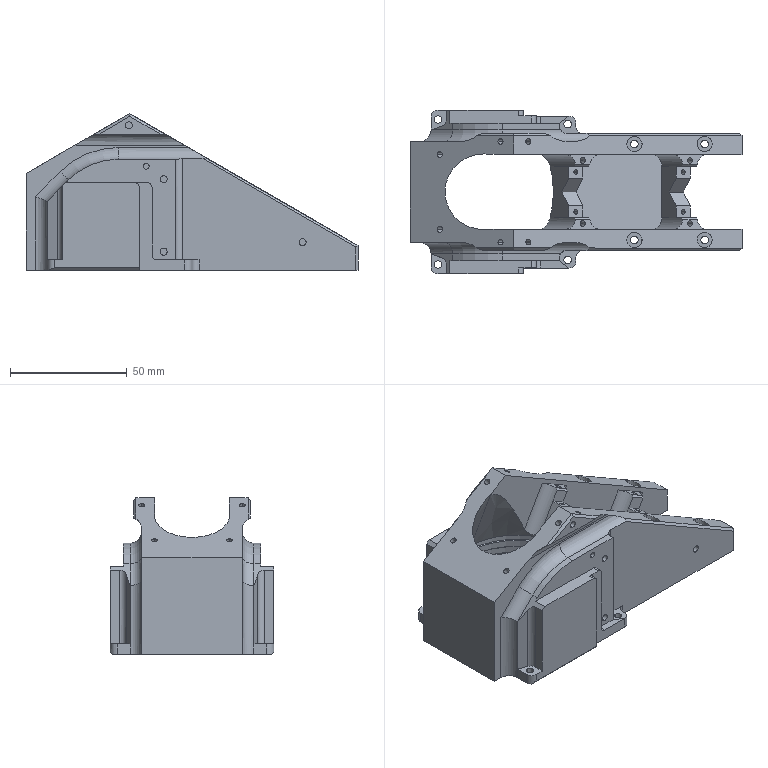NC program | NX | posted with a generic post | part box 142 x 70 x 67 mm
Lines 2969 to 4102 of 58889:
(PLANAR_MILL_COPY_COPY_COPY , TOOL : D6R0)
N5888 T04 M6
N5890 G54
N5892 G17 G0 G90 X-67.337 Y30.348 S3000 M3
N5894 G43 Z30. H4
N5896 G94 G1 Z-1. F5000.
N5898 G41 X-66.965 Y30.014 F1200. D4
N5900 G3 X-63.026 Y29.319 R4.
N5902 G1 X-58.5 Y30.966
N5904 Y35.
N5906 G3 X-60.5 Y38.464 R4.
N5908 G40
N5910 G1 X-60.941 Y38.699
N5912 G0 Z1.
N5914 X-67.337 Y30.348
N5916 G1 Z-2. F5000.
N5918 G41 X-66.965 Y30.014 F1200.
N5920 G3 X-63.026 Y29.319 R4.
N5922 G1 X-58.5 Y30.966
N5924 Y35.
N5926 G3 X-60.5 Y38.464 R4.
N5928 G40
N5930 G1 X-60.941 Y38.699
N5932 G0 Z0.
N5934 X-67.337 Y30.348
N5936 G1 Z-3. F5000.
N5938 G41 X-66.965 Y30.014 F1200.
N5940 G3 X-63.026 Y29.319 R4.
N5942 G1 X-58.5 Y30.966
N5944 Y35.
N5946 G3 X-60.5 Y38.464 R4.
N5948 G40
N5950 G1 X-60.941 Y38.699
N5952 G0 Z-1.
N5954 X-67.337 Y30.348
N5956 G1 Z-4. F5000.
N5958 G41 X-66.965 Y30.014 F1200.
N5960 G3 X-63.026 Y29.319 R4.
N5962 G1 X-58.5 Y30.966
N5964 Y35.
N5966 G3 X-60.5 Y38.464 R4.
N5968 G40
N5970 G1 X-60.941 Y38.699
N5972 G0 Z-2.
N5974 X-67.337 Y30.348
N5976 G1 Z-5. F5000.
N5978 G41 X-66.965 Y30.014 F1200.
N5980 G3 X-63.026 Y29.319 R4.
N5982 G1 X-58.5 Y30.966
N5984 Y35.
N5986 G3 X-60.5 Y38.464 R4.
N5988 G40
N5990 G1 X-60.941 Y38.699
N5992 G0 Z-3.
N5994 X-67.337 Y30.348
N5996 G1 Z-6. F5000.
N5998 G41 X-66.965 Y30.014 F1200.
N6000 G3 X-63.026 Y29.319 R4.
N6002 G1 X-58.5 Y30.966
N6004 Y35.
N6006 G3 X-60.5 Y38.464 R4.
N6008 G40
N6010 G1 X-60.941 Y38.699
N6012 G0 Z-4.
N6014 X-67.337 Y30.348
N6016 G1 Z-7. F5000.
N6018 G41 X-66.965 Y30.014 F1200.
N6020 G3 X-63.026 Y29.319 R4.
N6022 G1 X-58.5 Y30.966
N6024 Y35.
N6026 G3 X-60.5 Y38.464 R4.
N6028 G40
N6030 G1 X-60.941 Y38.699
N6032 G0 Z-5.
N6034 X-67.337 Y30.348
N6036 G1 Z-8. F5000.
N6038 G41 X-66.965 Y30.014 F1200.
N6040 G3 X-63.026 Y29.319 R4.
N6042 G1 X-58.5 Y30.966
N6044 Y35.
N6046 G3 X-60.5 Y38.464 R4.
N6048 G40
N6050 G1 X-60.941 Y38.699
N6052 G0 Z-6.
N6054 X-67.337 Y30.348
N6056 G1 Z-9. F5000.
N6058 G41 X-66.965 Y30.014 F1200.
N6060 G3 X-63.026 Y29.319 R4.
N6062 G1 X-58.5 Y30.966
N6064 Y35.
N6066 G3 X-60.5 Y38.464 R4.
N6068 G40
N6070 G1 X-60.941 Y38.699
N6072 G0 Z-7.
N6074 X-67.337 Y30.348
N6076 G1 Z-10. F5000.
N6078 G41 X-66.965 Y30.014 F1200.
N6080 G3 X-63.026 Y29.319 R4.
N6082 G1 X-58.5 Y30.966
N6084 Y35.
N6086 G3 X-60.5 Y38.464 R4.
N6088 G40
N6090 G1 X-60.941 Y38.699
N6092 G0 Z-8.
N6094 X-67.337 Y30.348
N6096 G1 Z-11. F5000.
N6098 G41 X-66.965 Y30.014 F1200.
N6100 G3 X-63.026 Y29.319 R4.
N6102 G1 X-58.5 Y30.966
N6104 Y35.
N6106 G3 X-60.5 Y38.464 R4.
N6108 G40
N6110 G1 X-60.941 Y38.699
N6112 G0 Z-9.
N6114 X-67.337 Y30.348
N6116 G1 Z-12. F5000.
N6118 G41 X-66.965 Y30.014 F1200.
N6120 G3 X-63.026 Y29.319 R4.
N6122 G1 X-58.5 Y30.966
N6124 Y35.
N6126 G3 X-60.5 Y38.464 R4.
N6128 G40
N6130 G1 X-60.941 Y38.699
N6132 G0 Z-10.
N6134 X-67.337 Y30.348
N6136 G1 Z-13. F5000.
N6138 G41 X-66.965 Y30.014 F1200.
N6140 G3 X-63.026 Y29.319 R4.
N6142 G1 X-58.5 Y30.966
N6144 Y35.
N6146 G3 X-60.5 Y38.464 R4.
N6148 G40
N6150 G1 X-60.941 Y38.699
N6152 G0 Z-11.
N6154 X-67.337 Y30.348
N6156 G1 Z-14. F5000.
N6158 G41 X-66.965 Y30.014 F1200.
N6160 G3 X-63.026 Y29.319 R4.
N6162 G1 X-58.5 Y30.966
N6164 Y35.
N6166 G3 X-60.5 Y38.464 R4.
N6168 G40
N6170 G1 X-60.941 Y38.699
N6172 G0 Z-12.
N6174 X-67.337 Y30.348
N6176 G1 Z-15. F5000.
N6178 G41 X-66.965 Y30.014 F1200.
N6180 G3 X-63.026 Y29.319 R4.
N6182 G1 X-58.5 Y30.966
N6184 Y35.
N6186 G3 X-60.5 Y38.464 R4.
N6188 G40
N6190 G1 X-60.941 Y38.699
N6192 G0 Z-13.
N6194 X-67.337 Y30.348
N6196 G1 Z-16. F5000.
N6198 G41 X-66.965 Y30.014 F1200.
N6200 G3 X-63.026 Y29.319 R4.
N6202 G1 X-58.5 Y30.966
N6204 Y35.
N6206 G3 X-60.5 Y38.464 R4.
N6208 G40
N6210 G1 X-60.941 Y38.699
N6212 G0 Z-14.
N6214 X-67.337 Y30.348
N6216 G1 Z-17. F5000.
N6218 G41 X-66.965 Y30.014 F1200.
N6220 G3 X-63.026 Y29.319 R4.
N6222 G1 X-58.5 Y30.966
N6224 Y35.
N6226 G3 X-60.5 Y38.464 R4.
N6228 G40
N6230 G1 X-60.941 Y38.699
N6232 G0 Z-15.
N6234 X-67.337 Y30.348
N6236 G1 Z-18. F5000.
N6238 G41 X-66.965 Y30.014 F1200.
N6240 G3 X-63.026 Y29.319 R4.
N6242 G1 X-58.5 Y30.966
N6244 Y35.
N6246 G3 X-60.5 Y38.464 R4.
N6248 G40
N6250 G1 X-60.941 Y38.699
N6252 G0 Z-16.
N6254 X-67.337 Y30.348
N6256 G1 Z-19. F5000.
N6258 G41 X-66.965 Y30.014 F1200.
N6260 G3 X-63.026 Y29.319 R4.
N6262 G1 X-58.5 Y30.966
N6264 Y35.
N6266 G3 X-60.5 Y38.464 R4.
N6268 G40
N6270 G1 X-60.941 Y38.699
N6272 G0 Z-17.
N6274 X-67.337 Y30.348
N6276 G1 Z-20. F5000.
N6278 G41 X-66.965 Y30.014 F1200.
N6280 G3 X-63.026 Y29.319 R4.
N6282 G1 X-58.5 Y30.966
N6284 Y35.
N6286 G3 X-60.5 Y38.464 R4.
N6288 G40
N6290 G1 X-60.941 Y38.699
N6292 G0 Z-18.
N6294 X-67.337 Y30.348
N6296 G1 Z-21. F5000.
N6298 G41 X-66.965 Y30.014 F1200.
N6300 G3 X-63.026 Y29.319 R4.
N6302 G1 X-58.5 Y30.966
N6304 Y35.
N6306 G3 X-60.5 Y38.464 R4.
N6308 G40
N6310 G1 X-60.941 Y38.699
N6312 G0 Z-19.
N6314 X-67.337 Y30.348
N6316 G1 Z-22. F5000.
N6318 G41 X-66.965 Y30.014 F1200.
N6320 G3 X-63.026 Y29.319 R4.
N6322 G1 X-58.5 Y30.966
N6324 Y35.
N6326 G3 X-60.5 Y38.464 R4.
N6328 G40
N6330 G1 X-60.941 Y38.699
N6332 G0 Z-20.
N6334 X-67.337 Y30.348
N6336 G1 Z-23. F5000.
N6338 G41 X-66.965 Y30.014 F1200.
N6340 G3 X-63.026 Y29.319 R4.
N6342 G1 X-58.5 Y30.966
N6344 Y35.
N6346 G3 X-60.5 Y38.464 R4.
N6348 G40
N6350 G1 X-60.941 Y38.699
N6352 G0 Z-21.
N6354 X-67.337 Y30.348
N6356 G1 Z-24. F5000.
N6358 G41 X-66.965 Y30.014 F1200.
N6360 G3 X-63.026 Y29.319 R4.
N6362 G1 X-58.5 Y30.966
N6364 Y35.
N6366 G3 X-60.5 Y38.464 R4.
N6368 G40
N6370 G1 X-60.941 Y38.699
N6372 G0 Z-22.
N6374 X-67.337 Y30.348
N6376 G1 Z-25. F5000.
N6378 G41 X-66.965 Y30.014 F1200.
N6380 G3 X-63.026 Y29.319 R4.
N6382 G1 X-58.5 Y30.966
N6384 Y35.
N6386 G3 X-60.5 Y38.464 R4.
N6388 G40
N6390 G1 X-60.941 Y38.699
N6392 G0 Z-23.
N6394 X-67.337 Y30.348
N6396 G1 Z-26. F5000.
N6398 G41 X-66.965 Y30.014 F1200.
N6400 G3 X-63.026 Y29.319 R4.
N6402 G1 X-58.5 Y30.966
N6404 Y35.
N6406 G3 X-60.5 Y38.464 R4.
N6408 G40
N6410 G1 X-60.941 Y38.699
N6412 G0 Z-24.
N6414 X-67.337 Y30.348
N6416 G1 Z-27. F5000.
N6418 G41 X-66.965 Y30.014 F1200.
N6420 G3 X-63.026 Y29.319 R4.
N6422 G1 X-58.5 Y30.966
N6424 Y35.
N6426 G3 X-60.5 Y38.464 R4.
N6428 G40
N6430 G1 X-60.941 Y38.699
N6432 G0 Z-25.
N6434 X-67.337 Y30.348
N6436 G1 Z-28. F5000.
N6438 G41 X-66.965 Y30.014 F1200.
N6440 G3 X-63.026 Y29.319 R4.
N6442 G1 X-58.5 Y30.966
N6444 Y35.
N6446 G3 X-60.5 Y38.464 R4.
N6448 G40
N6450 G1 X-60.941 Y38.699
N6452 G0 Z-26.
N6454 X-67.337 Y30.348
N6456 G1 Z-29. F5000.
N6458 G41 X-66.965 Y30.014 F1200.
N6460 G3 X-63.026 Y29.319 R4.
N6462 G1 X-58.5 Y30.966
N6464 Y35.
N6466 G3 X-60.5 Y38.464 R4.
N6468 G40
N6470 G1 X-60.941 Y38.699
N6472 G0 Z-27.
N6474 X-67.337 Y30.348
N6476 G1 Z-30. F5000.
N6478 G41 X-66.965 Y30.014 F1200.
N6480 G3 X-63.026 Y29.319 R4.
N6482 G1 X-58.5 Y30.966
N6484 Y35.
N6486 G3 X-60.5 Y38.464 R4.
N6488 G40
N6490 G1 X-60.941 Y38.699
N6492 G0 Z-28.
N6494 X-67.337 Y30.348
N6496 G1 Z-31. F5000.
N6498 G41 X-66.965 Y30.014 F1200.
N6500 G3 X-63.026 Y29.319 R4.
N6502 G1 X-58.5 Y30.966
N6504 Y35.
N6506 G3 X-60.5 Y38.464 R4.
N6508 G40
N6510 G1 X-60.941 Y38.699
N6512 G0 Z-29.
N6514 X-67.337 Y30.348
N6516 G1 Z-32. F5000.
N6518 G41 X-66.965 Y30.014 F1200.
N6520 G3 X-63.026 Y29.319 R4.
N6522 G1 X-58.5 Y30.966
N6524 Y35.
N6526 G3 X-60.5 Y38.464 R4.
N6528 G40
N6530 G1 X-60.941 Y38.699
N6532 G0 Z-30.
N6534 X-67.337 Y30.348
N6536 G1 Z-33. F5000.
N6538 G41 X-66.965 Y30.014 F1200.
N6540 G3 X-63.026 Y29.319 R4.
N6542 G1 X-58.5 Y30.966
N6544 Y35.
N6546 G3 X-60.5 Y38.464 R4.
N6548 G40
N6550 G1 X-60.941 Y38.699
N6552 G0 Z-31.
N6554 X-67.337 Y30.348
N6556 G1 Z-34. F5000.
N6558 G41 X-66.965 Y30.014 F1200.
N6560 G3 X-63.026 Y29.319 R4.
N6562 G1 X-58.5 Y30.966
N6564 Y35.
N6566 G3 X-60.5 Y38.464 R4.
N6568 G40
N6570 G1 X-60.941 Y38.699
N6572 G0 Z-32.
N6574 X-67.337 Y30.348
N6576 G1 Z-35. F5000.
N6578 G41 X-66.965 Y30.014 F1200.
N6580 G3 X-63.026 Y29.319 R4.
N6582 G1 X-58.5 Y30.966
N6584 Y35.
N6586 G3 X-60.5 Y38.464 R4.
N6588 G40
N6590 G1 X-60.941 Y38.699
N6592 G0 Z-33.
N6594 X-67.337 Y30.348
N6596 G1 Z-36. F5000.
N6598 G41 X-66.965 Y30.014 F1200.
N6600 G3 X-63.026 Y29.319 R4.
N6602 G1 X-58.5 Y30.966
N6604 Y35.
N6606 G3 X-60.5 Y38.464 R4.
N6608 G40
N6610 G1 X-60.941 Y38.699
N6612 G0 Z-34.
N6614 X-67.337 Y30.348
N6616 G1 Z-37. F5000.
N6618 G41 X-66.965 Y30.014 F1200.
N6620 G3 X-63.026 Y29.319 R4.
N6622 G1 X-58.5 Y30.966
N6624 Y35.
N6626 G3 X-60.5 Y38.464 R4.
N6628 G40
N6630 G1 X-60.941 Y38.699
N6632 G0 Z-35.
N6634 X-67.337 Y30.348
N6636 G1 Z-38. F5000.
N6638 G41 X-66.965 Y30.014 F1200.
N6640 G3 X-63.026 Y29.319 R4.
N6642 G1 X-58.5 Y30.966
N6644 Y35.
N6646 G3 X-60.5 Y38.464 R4.
N6648 G40
N6650 G1 X-60.941 Y38.699
N6652 G0 Z-36.
N6654 X-67.337 Y30.348
N6656 G1 Z-39. F5000.
N6658 G41 X-66.965 Y30.014 F1200.
N6660 G3 X-63.026 Y29.319 R4.
N6662 G1 X-58.5 Y30.966
N6664 Y35.
N6666 G3 X-60.5 Y38.464 R4.
N6668 G40
N6670 G1 X-60.941 Y38.699
N6672 G0 Z-37.
N6674 X-67.337 Y30.348
N6676 G1 Z-40. F5000.
N6678 G41 X-66.965 Y30.014 F1200.
N6680 G3 X-63.026 Y29.319 R4.
N6682 G1 X-58.5 Y30.966
N6684 Y35.
N6686 G3 X-60.5 Y38.464 R4.
N6688 G40
N6690 G1 X-60.941 Y38.699
N6692 G0 Z-38.
N6694 X-67.337 Y30.348
N6696 G1 Z-41. F5000.
N6698 G41 X-66.965 Y30.014 F1200.
N6700 G3 X-63.026 Y29.319 R4.
N6702 G1 X-58.5 Y30.966
N6704 Y35.
N6706 G3 X-60.5 Y38.464 R4.
N6708 G40
N6710 G1 X-60.941 Y38.699
N6712 G0 Z-39.
N6714 X-67.337 Y30.348
N6716 G1 Z-42. F5000.
N6718 G41 X-66.965 Y30.014 F1200.
N6720 G3 X-63.026 Y29.319 R4.
N6722 G1 X-58.5 Y30.966
N6724 Y35.
N6726 G3 X-60.5 Y38.464 R4.
N6728 G40
N6730 G1 X-60.941 Y38.699
N6732 G0 Z-40.
N6734 X-67.337 Y30.348
N6736 G1 Z-43. F5000.
N6738 G41 X-66.965 Y30.014 F1200.
N6740 G3 X-63.026 Y29.319 R4.
N6742 G1 X-58.5 Y30.966
N6744 Y35.
N6746 G3 X-60.5 Y38.464 R4.
N6748 G40
N6750 G1 X-60.941 Y38.699
N6752 G0 Z-41.
N6754 X-67.337 Y30.348
N6756 G1 Z-44. F5000.
N6758 G41 X-66.965 Y30.014 F1200.
N6760 G3 X-63.026 Y29.319 R4.
N6762 G1 X-58.5 Y30.966
N6764 Y35.
N6766 G3 X-60.5 Y38.464 R4.
N6768 G40
N6770 G1 X-60.941 Y38.699
N6772 G0 Z-42.
N6774 X-67.337 Y30.348
N6776 G1 Z-45. F5000.
N6778 G41 X-66.965 Y30.014 F1200.
N6780 G3 X-63.026 Y29.319 R4.
N6782 G1 X-58.5 Y30.966
N6784 Y35.
N6786 G3 X-60.5 Y38.464 R4.
N6788 G40
N6790 G1 X-60.941 Y38.699
N6792 G0 Z-43.
N6794 X-67.337 Y30.348
N6796 G1 Z-46. F5000.
N6798 G41 X-66.965 Y30.014 F1200.
N6800 G3 X-63.026 Y29.319 R4.
N6802 G1 X-58.5 Y30.966
N6804 Y35.
N6806 G3 X-60.5 Y38.464 R4.
N6808 G40
N6810 G1 X-60.941 Y38.699
N6812 G0 Z-44.
N6814 X-67.337 Y30.348
N6816 G1 Z-47. F5000.
N6818 G41 X-66.965 Y30.014 F1200.
N6820 G3 X-63.026 Y29.319 R4.
N6822 G1 X-58.5 Y30.966
N6824 Y35.
N6826 G3 X-60.5 Y38.464 R4.
N6828 G40
N6830 G1 X-60.941 Y38.699
N6832 G0 Z-45.
N6834 X-67.337 Y30.348
N6836 G1 Z-48. F5000.
N6838 G41 X-66.965 Y30.014 F1200.
N6840 G3 X-63.026 Y29.319 R4.
N6842 G1 X-58.5 Y30.966
N6844 Y35.
N6846 G3 X-60.5 Y38.464 R4.
N6848 G40
N6850 G1 X-60.941 Y38.699
N6852 G0 Z-46.
N6854 X-67.337 Y30.348
N6856 G1 Z-49. F5000.
N6858 G41 X-66.965 Y30.014 F1200.
N6860 G3 X-63.026 Y29.319 R4.
N6862 G1 X-58.5 Y30.966
N6864 Y35.
N6866 G3 X-60.5 Y38.464 R4.
N6868 G40
N6870 G1 X-60.941 Y38.699
N6872 G0 Z-47.
N6874 X-67.337 Y30.348
N6876 G1 Z-50. F5000.
N6878 G41 X-66.965 Y30.014 F1200.
N6880 G3 X-63.026 Y29.319 R4.
N6882 G1 X-58.5 Y30.966
N6884 Y35.
N6886 G3 X-60.5 Y38.464 R4.
N6888 G40
N6890 G1 X-60.941 Y38.699
N6892 G0 Z-48.
N6894 X-67.337 Y30.348
N6896 G1 Z-51. F5000.
N6898 G41 X-66.965 Y30.014 F1200.
N6900 G3 X-63.026 Y29.319 R4.
N6902 G1 X-58.5 Y30.966
N6904 Y35.
N6906 G3 X-60.5 Y38.464 R4.
N6908 G40
N6910 G1 X-60.941 Y38.699
N6912 G0 Z-49.
N6914 X-67.337 Y30.348
N6916 G1 Z-52. F5000.
N6918 G41 X-66.965 Y30.014 F1200.
N6920 G3 X-63.026 Y29.319 R4.
N6922 G1 X-58.5 Y30.966
N6924 Y35.
N6926 G3 X-60.5 Y38.464 R4.
N6928 G40
N6930 G1 X-60.941 Y38.699
N6932 G0 Z-50.
N6934 X-67.337 Y30.348
N6936 G1 Z-53. F5000.
N6938 G41 X-66.965 Y30.014 F1200.
N6940 G3 X-63.026 Y29.319 R4.
N6942 G1 X-58.5 Y30.966
N6944 Y35.
N6946 G3 X-60.5 Y38.464 R4.
N6948 G40
N6950 G1 X-60.941 Y38.699
N6952 G0 Z-51.
N6954 X-67.337 Y30.348
N6956 G1 Z-54. F5000.
N6958 G41 X-66.965 Y30.014 F1200.
N6960 G3 X-63.026 Y29.319 R4.
N6962 G1 X-58.5 Y30.966
N6964 Y35.
N6966 G3 X-60.5 Y38.464 R4.
N6968 G40
N6970 G1 X-60.941 Y38.699
N6972 G0 Z-52.
N6974 X-67.337 Y30.348
N6976 G1 Z-55. F5000.
N6978 G41 X-66.965 Y30.014 F1200.
N6980 G3 X-63.026 Y29.319 R4.
N6982 G1 X-58.5 Y30.966
N6984 Y35.
N6986 G3 X-60.5 Y38.464 R4.
N6988 G40
N6990 G1 X-60.941 Y38.699
N6992 G0 Z-53.
N6994 X-67.337 Y30.348
N6996 G1 Z-56. F5000.
N6998 G41 X-66.965 Y30.014 F1200.
N7000 G3 X-63.026 Y29.319 R4.
N7002 G1 X-58.5 Y30.966
N7004 Y35.
N7006 G3 X-60.5 Y38.464 R4.
N7008 G40
N7010 G1 X-60.941 Y38.699
N7012 G0 Z-54.
N7014 X-67.337 Y30.348
N7016 G1 Z-57. F5000.
N7018 G41 X-66.965 Y30.014 F1200.
N7020 G3 X-63.026 Y29.319 R4.
N7022 G1 X-58.5 Y30.966
N7024 Y35.
N7026 G3 X-60.5 Y38.464 R4.
N7028 G40
N7030 G1 X-60.941 Y38.699
N7032 G0 Z-55.
N7034 X-67.337 Y30.348
N7036 G1 Z-58. F5000.
N7038 G41 X-66.965 Y30.014 F1200.
N7040 G3 X-63.026 Y29.319 R4.
N7042 G1 X-58.5 Y30.966
N7044 Y35.
N7046 G3 X-60.5 Y38.464 R4.
N7048 G40
N7050 G1 X-60.941 Y38.699
N7052 G0 Z-56.
N7054 X-67.337 Y30.348
N7056 G1 Z-59. F5000.
N7058 G41 X-66.965 Y30.014 F1200.
N7060 G3 X-63.026 Y29.319 R4.
N7062 G1 X-58.5 Y30.966
N7064 Y35.
N7066 G3 X-60.5 Y38.464 R4.
N7068 G40
N7070 G1 X-60.941 Y38.699
N7072 G0 Z-57.
N7074 X-67.337 Y30.348
N7076 G1 Z-60. F5000.
N7078 G41 X-66.965 Y30.014 F1200.
N7080 G3 X-63.026 Y29.319 R4.
N7082 G1 X-58.5 Y30.966
N7084 Y35.
N7086 G3 X-60.5 Y38.464 R4.
N7088 G40
N7090 G1 X-60.941 Y38.699
N7092 G0 Z-58.
N7094 X-67.337 Y30.348
N7096 G1 Z-61. F5000.
N7098 G41 X-66.965 Y30.014 F1200.
N7100 G3 X-63.026 Y29.319 R4.
N7102 G1 X-58.5 Y30.966
N7104 Y35.
N7106 G3 X-60.5 Y38.464 R4.
N7108 G40
N7110 G1 X-60.941 Y38.699
N7112 G0 Z-59.
N7114 X-67.337 Y30.348
N7116 G1 Z-62. F5000.
N7118 G41 X-66.965 Y30.014 F1200.
N7120 G3 X-63.026 Y29.319 R4.
N7122 G1 X-58.5 Y30.966
N7124 Y35.
N7126 G3 X-60.5 Y38.464 R4.
N7128 G40
N7130 G1 X-60.941 Y38.699
N7132 G0 Z-60.
N7134 X-67.337 Y30.348
N7136 G1 Z-62.5 F5000.
N7138 G41 X-66.965 Y30.014 F1200.
N7140 G3 X-63.026 Y29.319 R4.
N7142 G1 X-58.5 Y30.966
N7144 Y35.
N7146 G3 X-60.5 Y38.464 R4.
N7148 G40
N7150 G1 X-60.941 Y38.699
N7152 G0 Z30.
N7154 X-1.659 Y36.199
N7156 G1 Z-1. F5000.
N7158 G41 X-2.1 Y35.964 F1200.
N7160 G3 X-4.1 Y32.5 R4.
N7162 G1 Y28.
N7164 X4.
N7166 G3 X7.464 Y30. R4.
N7168 G40
N7170 G1 X7.699 Y30.441
N7172 G0 Z1.
N7174 X-1.659 Y36.199
N7176 G1 Z-2. F5000.
N7178 G41 X-2.1 Y35.964 F1200.
N7180 G3 X-4.1 Y32.5 R4.
N7182 G1 Y28.
N7184 X4.
N7186 G3 X7.464 Y30. R4.
N7188 G40
N7190 G1 X7.699 Y30.441
N7192 G0 Z0.
N7194 X-1.659 Y36.199
N7196 G1 Z-3. F5000.
N7198 G41 X-2.1 Y35.964 F1200.
N7200 G3 X-4.1 Y32.5 R4.
N7202 G1 Y28.
N7204 X4.
N7206 G3 X7.464 Y30. R4.
N7208 G40
N7210 G1 X7.699 Y30.441
N7212 G0 Z-1.
N7214 X-1.659 Y36.199
N7216 G1 Z-4. F5000.
N7218 G41 X-2.1 Y35.964 F1200.
N7220 G3 X-4.1 Y32.5 R4.
N7222 G1 Y28.
N7224 X4.
N7226 G3 X7.464 Y30. R4.
N7228 G40
N7230 G1 X7.699 Y30.441
N7232 G0 Z-2.
N7234 X-1.659 Y36.199
N7236 G1 Z-5. F5000.
N7238 G41 X-2.1 Y35.964 F1200.
N7240 G3 X-4.1 Y32.5 R4.
N7242 G1 Y28.
N7244 X4.
N7246 G3 X7.464 Y30. R4.
N7248 G40
N7250 G1 X7.699 Y30.441
N7252 G0 Z-3.
N7254 X-1.659 Y36.199
N7256 G1 Z-6. F5000.
N7258 G41 X-2.1 Y35.964 F1200.
N7260 G3 X-4.1 Y32.5 R4.
N7262 G1 Y28.
N7264 X4.
N7266 G3 X7.464 Y30. R4.
N7268 G40
N7270 G1 X7.699 Y30.441
N7272 G0 Z-4.
N7274 X-1.659 Y36.199
N7276 G1 Z-7. F5000.
N7278 G41 X-2.1 Y35.964 F1200.
N7280 G3 X-4.1 Y32.5 R4.
N7282 G1 Y28.
N7284 X4.
N7286 G3 X7.464 Y30. R4.
N7288 G40
N7290 G1 X7.699 Y30.441
N7292 G0 Z-5.
N7294 X-1.659 Y36.199
N7296 G1 Z-8. F5000.
N7298 G41 X-2.1 Y35.964 F1200.
N7300 G3 X-4.1 Y32.5 R4.
N7302 G1 Y28.
N7304 X4.
N7306 G3 X7.464 Y30. R4.
N7308 G40
N7310 G1 X7.699 Y30.441
N7312 G0 Z-6.
N7314 X-1.659 Y36.199
N7316 G1 Z-9. F5000.
N7318 G41 X-2.1 Y35.964 F1200.
N7320 G3 X-4.1 Y32.5 R4.
N7322 G1 Y28.
N7324 X4.
N7326 G3 X7.464 Y30. R4.
N7328 G40
N7330 G1 X7.699 Y30.441
N7332 G0 Z-7.
N7334 X-1.659 Y36.199
N7336 G1 Z-10. F5000.
N7338 G41 X-2.1 Y35.964 F1200.
N7340 G3 X-4.1 Y32.5 R4.
N7342 G1 Y28.
N7344 X4.
N7346 G3 X7.464 Y30. R4.
N7348 G40
N7350 G1 X7.699 Y30.441
N7352 G0 Z-8.
N7354 X-1.659 Y36.199
N7356 G1 Z-11. F5000.
N7358 G41 X-2.1 Y35.964 F1200.
N7360 G3 X-4.1 Y32.5 R4.
N7362 G1 Y28.
N7364 X4.
N7366 G3 X7.464 Y30. R4.
N7368 G40
N7370 G1 X7.699 Y30.441
N7372 G0 Z-9.
N7374 X-1.659 Y36.199
N7376 G1 Z-12. F5000.
N7378 G41 X-2.1 Y35.964 F1200.
N7380 G3 X-4.1 Y32.5 R4.
N7382 G1 Y28.
N7384 X4.
N7386 G3 X7.464 Y30. R4.
N7388 G40
N7390 G1 X7.699 Y30.441
N7392 G0 Z-10.
N7394 X-1.659 Y36.199
N7396 G1 Z-13. F5000.
N7398 G41 X-2.1 Y35.964 F1200.
N7400 G3 X-4.1 Y32.5 R4.
N7402 G1 Y28.
N7404 X4.
N7406 G3 X7.464 Y30. R4.
N7408 G40
N7410 G1 X7.699 Y30.441
N7412 G0 Z-11.
N7414 X-1.659 Y36.199
N7416 G1 Z-14. F5000.
N7418 G41 X-2.1 Y35.964 F1200.
N7420 G3 X-4.1 Y32.5 R4.
N7422 G1 Y28.
N7424 X4.
N7426 G3 X7.464 Y30. R4.
N7428 G40
N7430 G1 X7.699 Y30.441
N7432 G0 Z-12.
N7434 X-1.659 Y36.199
N7436 G1 Z-15. F5000.
N7438 G41 X-2.1 Y35.964 F1200.
N7440 G3 X-4.1 Y32.5 R4.
N7442 G1 Y28.
N7444 X4.
N7446 G3 X7.464 Y30. R4.
N7448 G40
N7450 G1 X7.699 Y30.441
N7452 G0 Z-13.
N7454 X-1.659 Y36.199
N7456 G1 Z-16. F5000.
N7458 G41 X-2.1 Y35.964 F1200.
N7460 G3 X-4.1 Y32.5 R4.
N7462 G1 Y28.
N7464 X4.
N7466 G3 X7.464 Y30. R4.
N7468 G40
N7470 G1 X7.699 Y30.441
N7472 G0 Z-14.
N7474 X-1.659 Y36.199
N7476 G1 Z-17. F5000.
N7478 G41 X-2.1 Y35.964 F1200.
N7480 G3 X-4.1 Y32.5 R4.
N7482 G1 Y28.
N7484 X4.
N7486 G3 X7.464 Y30. R4.
N7488 G40
N7490 G1 X7.699 Y30.441
N7492 G0 Z-15.
N7494 X-1.659 Y36.199
N7496 G1 Z-18. F5000.
N7498 G41 X-2.1 Y35.964 F1200.
N7500 G3 X-4.1 Y32.5 R4.
N7502 G1 Y28.
N7504 X4.
N7506 G3 X7.464 Y30. R4.
N7508 G40
N7510 G1 X7.699 Y30.441
N7512 G0 Z-16.
N7514 X-1.659 Y36.199
N7516 G1 Z-19. F5000.
N7518 G41 X-2.1 Y35.964 F1200.
N7520 G3 X-4.1 Y32.5 R4.
N7522 G1 Y28.
N7524 X4.
N7526 G3 X7.464 Y30. R4.
N7528 G40
N7530 G1 X7.699 Y30.441
N7532 G0 Z-17.
N7534 X-1.659 Y36.199
N7536 G1 Z-20. F5000.
N7538 G41 X-2.1 Y35.964 F1200.
N7540 G3 X-4.1 Y32.5 R4.
N7542 G1 Y28.
N7544 X4.
N7546 G3 X7.464 Y30. R4.
N7548 G40
N7550 G1 X7.699 Y30.441
N7552 G0 Z-18.
N7554 X-1.659 Y36.199
N7556 G1 Z-21. F5000.
N7558 G41 X-2.1 Y35.964 F1200.
N7560 G3 X-4.1 Y32.5 R4.
N7562 G1 Y28.
N7564 X4.
N7566 G3 X7.464 Y30. R4.
N7568 G40
N7570 G1 X7.699 Y30.441
N7572 G0 Z-19.
N7574 X-1.659 Y36.199
N7576 G1 Z-22. F5000.
N7578 G41 X-2.1 Y35.964 F1200.
N7580 G3 X-4.1 Y32.5 R4.
N7582 G1 Y28.
N7584 X4.
N7586 G3 X7.464 Y30. R4.
N7588 G40
N7590 G1 X7.699 Y30.441
N7592 G0 Z-20.
N7594 X-1.659 Y36.199
N7596 G1 Z-23. F5000.
N7598 G41 X-2.1 Y35.964 F1200.
N7600 G3 X-4.1 Y32.5 R4.
N7602 G1 Y28.
N7604 X4.
N7606 G3 X7.464 Y30. R4.
N7608 G40
N7610 G1 X7.699 Y30.441
N7612 G0 Z-21.
N7614 X-1.659 Y36.199
N7616 G1 Z-24. F5000.
N7618 G41 X-2.1 Y35.964 F1200.
N7620 G3 X-4.1 Y32.5 R4.
N7622 G1 Y28.
N7624 X4.
N7626 G3 X7.464 Y30. R4.
N7628 G40
N7630 G1 X7.699 Y30.441
N7632 G0 Z-22.
N7634 X-1.659 Y36.199
N7636 G1 Z-25. F5000.
N7638 G41 X-2.1 Y35.964 F1200.
N7640 G3 X-4.1 Y32.5 R4.
N7642 G1 Y28.
N7644 X4.
N7646 G3 X7.464 Y30. R4.
N7648 G40
N7650 G1 X7.699 Y30.441
N7652 G0 Z-23.
N7654 X-1.659 Y36.199
N7656 G1 Z-26. F5000.
N7658 G41 X-2.1 Y35.964 F1200.
N7660 G3 X-4.1 Y32.5 R4.
N7662 G1 Y28.
N7664 X4.
N7666 G3 X7.464 Y30. R4.
N7668 G40
N7670 G1 X7.699 Y30.441
N7672 G0 Z-24.
N7674 X-1.659 Y36.199
N7676 G1 Z-27. F5000.
N7678 G41 X-2.1 Y35.964 F1200.
N7680 G3 X-4.1 Y32.5 R4.
N7682 G1 Y28.
N7684 X4.
N7686 G3 X7.464 Y30. R4.
N7688 G40
N7690 G1 X7.699 Y30.441
N7692 G0 Z-25.
N7694 X-1.659 Y36.199
N7696 G1 Z-28. F5000.
N7698 G41 X-2.1 Y35.964 F1200.
N7700 G3 X-4.1 Y32.5 R4.
N7702 G1 Y28.
N7704 X4.
N7706 G3 X7.464 Y30. R4.
N7708 G40
N7710 G1 X7.699 Y30.441
N7712 G0 Z-26.
N7714 X-1.659 Y36.199
N7716 G1 Z-29. F5000.
N7718 G41 X-2.1 Y35.964 F1200.
N7720 G3 X-4.1 Y32.5 R4.
N7722 G1 Y28.
N7724 X4.
N7726 G3 X7.464 Y30. R4.
N7728 G40
N7730 G1 X7.699 Y30.441
N7732 G0 Z-27.
N7734 X-1.659 Y36.199
N7736 G1 Z-30. F5000.
N7738 G41 X-2.1 Y35.964 F1200.
N7740 G3 X-4.1 Y32.5 R4.
N7742 G1 Y28.
N7744 X4.
N7746 G3 X7.464 Y30. R4.
N7748 G40
N7750 G1 X7.699 Y30.441
N7752 G0 Z-28.
N7754 X-1.659 Y36.199
N7756 G1 Z-31. F5000.
N7758 G41 X-2.1 Y35.964 F1200.
N7760 G3 X-4.1 Y32.5 R4.
N7762 G1 Y28.
N7764 X4.
N7766 G3 X7.464 Y30. R4.
N7768 G40
N7770 G1 X7.699 Y30.441
N7772 G0 Z-29.
N7774 X-1.659 Y36.199
N7776 G1 Z-32. F5000.
N7778 G41 X-2.1 Y35.964 F1200.
N7780 G3 X-4.1 Y32.5 R4.
N7782 G1 Y28.
N7784 X4.
N7786 G3 X7.464 Y30. R4.
N7788 G40
N7790 G1 X7.699 Y30.441
N7792 G0 Z-30.
N7794 X-1.659 Y36.199
N7796 G1 Z-33. F5000.
N7798 G41 X-2.1 Y35.964 F1200.
N7800 G3 X-4.1 Y32.5 R4.
N7802 G1 Y28.
N7804 X4.
N7806 G3 X7.464 Y30. R4.
N7808 G40
N7810 G1 X7.699 Y30.441
N7812 G0 Z-31.
N7814 X-1.659 Y36.199
N7816 G1 Z-34. F5000.
N7818 G41 X-2.1 Y35.964 F1200.
N7820 G3 X-4.1 Y32.5 R4.
N7822 G1 Y28.
N7824 X4.
N7826 G3 X7.464 Y30. R4.
N7828 G40
N7830 G1 X7.699 Y30.441
N7832 G0 Z-32.
N7834 X-1.659 Y36.199
N7836 G1 Z-35. F5000.
N7838 G41 X-2.1 Y35.964 F1200.
N7840 G3 X-4.1 Y32.5 R4.
N7842 G1 Y28.
N7844 X4.
N7846 G3 X7.464 Y30. R4.
N7848 G40
N7850 G1 X7.699 Y30.441
N7852 G0 Z-33.
N7854 X-1.659 Y36.199
N7856 G1 Z-36. F5000.
N7858 G41 X-2.1 Y35.964 F1200.
N7860 G3 X-4.1 Y32.5 R4.
N7862 G1 Y28.
N7864 X4.
N7866 G3 X7.464 Y30. R4.
N7868 G40
N7870 G1 X7.699 Y30.441
N7872 G0 Z-34.
N7874 X-1.659 Y36.199
N7876 G1 Z-37. F5000.
N7878 G41 X-2.1 Y35.964 F1200.
N7880 G3 X-4.1 Y32.5 R4.
N7882 G1 Y28.
N7884 X4.
N7886 G3 X7.464 Y30. R4.
N7888 G40
N7890 G1 X7.699 Y30.441
N7892 G0 Z-35.
N7894 X-1.659 Y36.199
N7896 G1 Z-38. F5000.
N7898 G41 X-2.1 Y35.964 F1200.
N7900 G3 X-4.1 Y32.5 R4.
N7902 G1 Y28.
N7904 X4.
N7906 G3 X7.464 Y30. R4.
N7908 G40
N7910 G1 X7.699 Y30.441
N7912 G0 Z-36.
N7914 X-1.659 Y36.199
N7916 G1 Z-39. F5000.
N7918 G41 X-2.1 Y35.964 F1200.
N7920 G3 X-4.1 Y32.5 R4.
N7922 G1 Y28.
N7924 X4.
N7926 G3 X7.464 Y30. R4.
N7928 G40
N7930 G1 X7.699 Y30.441
N7932 G0 Z-37.
N7934 X-1.659 Y36.199
N7936 G1 Z-40. F5000.
N7938 G41 X-2.1 Y35.964 F1200.
N7940 G3 X-4.1 Y32.5 R4.
N7942 G1 Y28.
N7944 X4.
N7946 G3 X7.464 Y30. R4.
N7948 G40
N7950 G1 X7.699 Y30.441
N7952 G0 Z-38.
N7954 X-1.659 Y36.199
N7956 G1 Z-41. F5000.
N7958 G41 X-2.1 Y35.964 F1200.
N7960 G3 X-4.1 Y32.5 R4.
N7962 G1 Y28.
N7964 X4.
N7966 G3 X7.464 Y30. R4.
N7968 G40
N7970 G1 X7.699 Y30.441
N7972 G0 Z-39.
N7974 X-1.659 Y36.199
N7976 G1 Z-42. F5000.
N7978 G41 X-2.1 Y35.964 F1200.
N7980 G3 X-4.1 Y32.5 R4.
N7982 G1 Y28.
N7984 X4.
N7986 G3 X7.464 Y30. R4.
N7988 G40
N7990 G1 X7.699 Y30.441
N7992 G0 Z-40.
N7994 X-1.659 Y36.199
N7996 G1 Z-43. F5000.
N7998 G41 X-2.1 Y35.964 F1200.
N8000 G3 X-4.1 Y32.5 R4.
N8002 G1 Y28.
N8004 X4.
N8006 G3 X7.464 Y30. R4.
N8008 G40
N8010 G1 X7.699 Y30.441
N8012 G0 Z-41.
N8014 X-1.659 Y36.199
N8016 G1 Z-44. F5000.
N8018 G41 X-2.1 Y35.964 F1200.
N8020 G3 X-4.1 Y32.5 R4.
N8022 G1 Y28.
N8024 X4.
N8026 G3 X7.464 Y30. R4.
N8028 G40
N8030 G1 X7.699 Y30.441
N8032 G0 Z-42.
N8034 X-1.659 Y36.199
N8036 G1 Z-45. F5000.
N8038 G41 X-2.1 Y35.964 F1200.
N8040 G3 X-4.1 Y32.5 R4.
N8042 G1 Y28.
N8044 X4.
N8046 G3 X7.464 Y30. R4.
N8048 G40
N8050 G1 X7.699 Y30.441
N8052 G0 Z-43.
N8054 X-1.659 Y36.199
N8056 G1 Z-46. F5000.
N8058 G41 X-2.1 Y35.964 F1200.
N8060 G3 X-4.1 Y32.5 R4.
N8062 G1 Y28.
N8064 X4.
N8066 G3 X7.464 Y30. R4.
N8068 G40
N8070 G1 X7.699 Y30.441
N8072 G0 Z-44.
N8074 X-1.659 Y36.199
N8076 G1 Z-47. F5000.
N8078 G41 X-2.1 Y35.964 F1200.
N8080 G3 X-4.1 Y32.5 R4.
N8082 G1 Y28.
N8084 X4.
N8086 G3 X7.464 Y30. R4.
N8088 G40
N8090 G1 X7.699 Y30.441
N8092 G0 Z-45.
N8094 X-1.659 Y36.199
N8096 G1 Z-48. F5000.
N8098 G41 X-2.1 Y35.964 F1200.
N8100 G3 X-4.1 Y32.5 R4.
N8102 G1 Y28.
N8104 X4.
N8106 G3 X7.464 Y30. R4.
N8108 G40
N8110 G1 X7.699 Y30.441
N8112 G0 Z-46.
N8114 X-1.659 Y36.199
N8116 G1 Z-49. F5000.
N8118 G41 X-2.1 Y35.964 F1200.
N8120 G3 X-4.1 Y32.5 R4.
N8122 G1 Y28.
N8124 X4.
N8126 G3 X7.464 Y30. R4.
N8128 G40
N8130 G1 X7.699 Y30.441
N8132 G0 Z-47.
N8134 X-1.659 Y36.199
N8136 G1 Z-50. F5000.
N8138 G41 X-2.1 Y35.964 F1200.
N8140 G3 X-4.1 Y32.5 R4.
N8142 G1 Y28.
N8144 X4.
N8146 G3 X7.464 Y30. R4.
N8148 G40